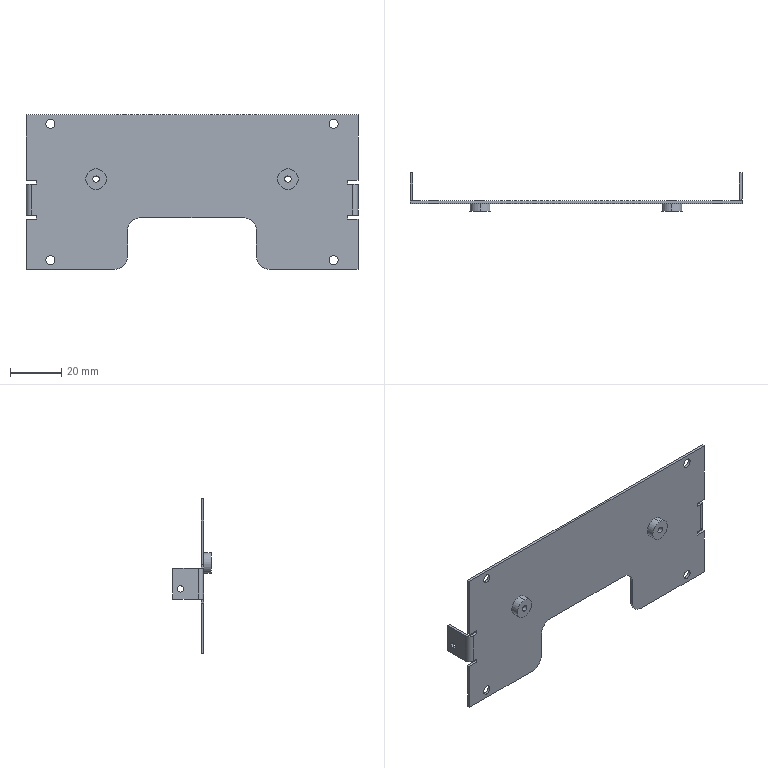Part | SolidWorks | features BaseBody 1 | 1 solid | 66 faces | box 129 x 15 x 60 mm | volume 7169 mm3 | plane 34 | cylinder 32 | commonest cylinder face diameters 3.5 x12 2.5 x8 8 x4 10 x4 2 x2 4 x2